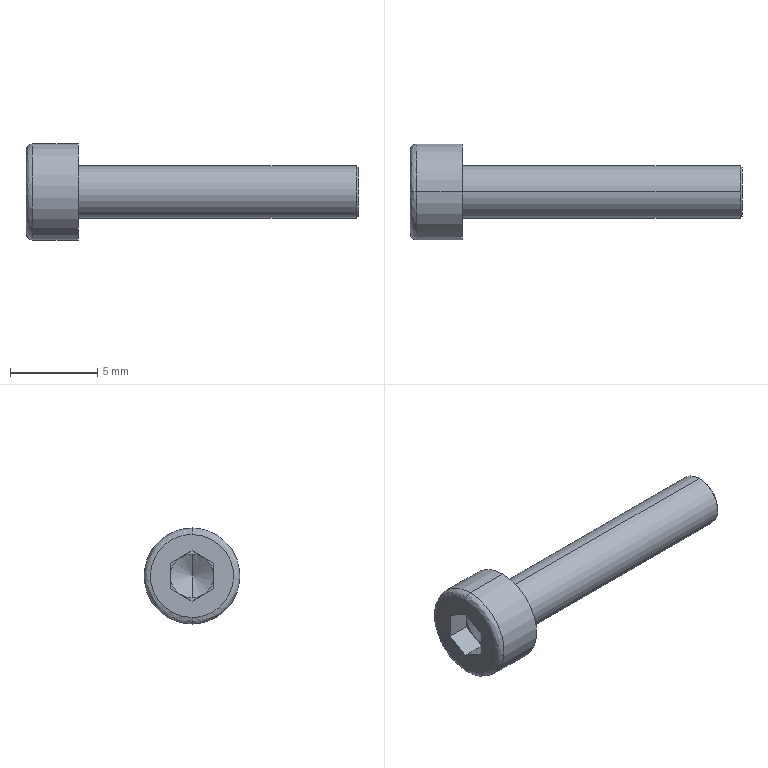Part | STEP file | hexagon socket head cap screws_gb_GB_FASTENER_SCREWS_HSHCS M3X16-N | 1 solid | 25 faces | box 19 x 5.5 x 5.5 mm | volume 175.607 mm3 | plane 15 | cylinder 4 | cone 4 | spline 2 | commonest cylinder face diameters 3 x2 5.5 x2